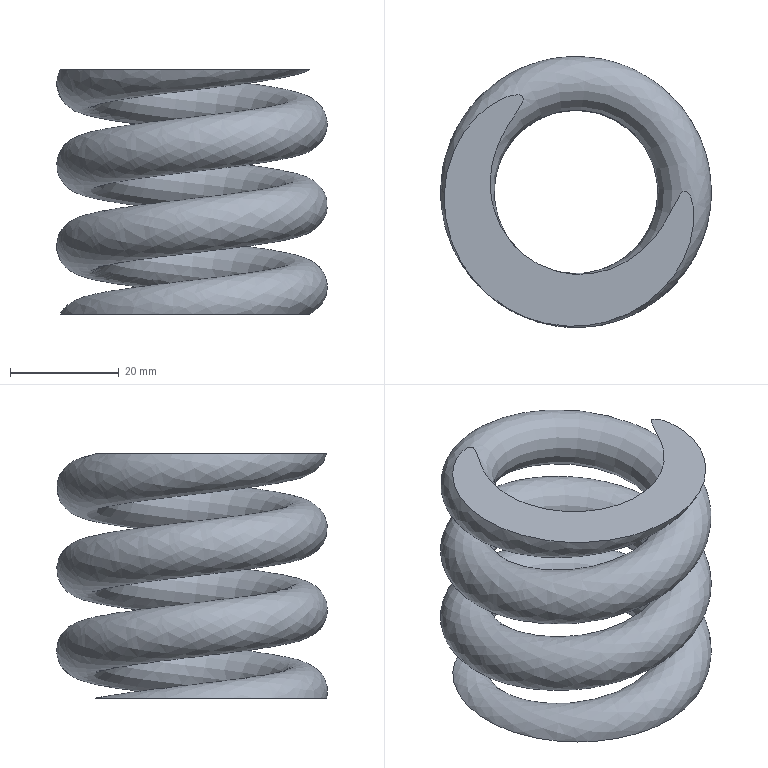Part | NX | features solid 2 | 1 solid | 3 faces | volume 28639 mm3 | plane 2 | spline 1